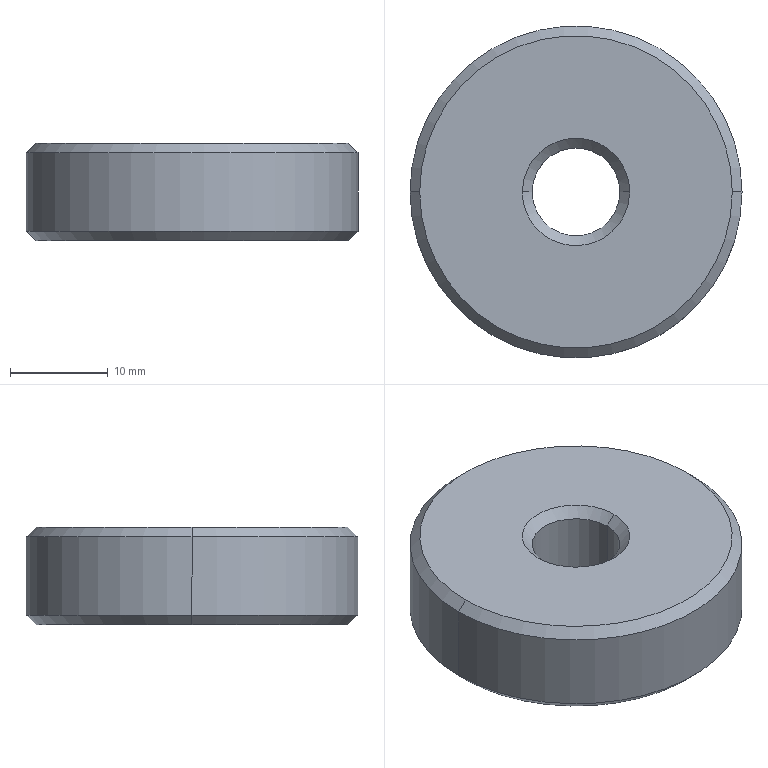Part | STEP file | 101000007785 | 1 solid | 14 faces | box 34 x 34 x 10 mm | volume 8308 mm3 | cone 8 | cylinder 4 | plane 2 | commonest cylinder face diameters 9 x2 34 x2
STEP:
#1=CARTESIAN_POINT('',(16.,0.,10.));
#2=VERTEX_POINT('',#1);
#3=CARTESIAN_POINT('',(-16.,0.,10.));
#4=VERTEX_POINT('',#3);
#5=CARTESIAN_POINT('',(0.,0.,10.));
#6=DIRECTION('',(0.,0.,-1.));
#7=AXIS2_PLACEMENT_3D('',#5,#6,$);
#8=CIRCLE('',#7,16.);
#9=EDGE_CURVE('',#2,#4,#8,.F.);
#10=ORIENTED_EDGE('',*,*,#9,.F.);
#11=CARTESIAN_POINT('',(17.,0.,9.));
#12=VERTEX_POINT('',#11);
#13=CARTESIAN_POINT('',(353561.391,0.,-353535.391));
#14=DIRECTION('',(0.7071,0.,-0.7071));
#15=VECTOR('',#14,1.);
#16=LINE('',#13,#15);
#17=EDGE_CURVE('',#2,#12,#16,.T.);
#18=ORIENTED_EDGE('',*,*,#17,.T.);
#19=CARTESIAN_POINT('',(-17.,0.,9.));
#20=VERTEX_POINT('',#19);
#21=CARTESIAN_POINT('',(0.,0.,9.));
#22=DIRECTION('',(0.,0.,-1.));
#23=AXIS2_PLACEMENT_3D('',#21,#22,$);
#24=CIRCLE('',#23,17.);
#25=EDGE_CURVE('',#20,#12,#24,.T.);
#26=ORIENTED_EDGE('',*,*,#25,.F.);
#27=CARTESIAN_POINT('',(-353561.391,0.,-353535.391));
#28=DIRECTION('',(-0.7071,0.,-0.7071));
#29=VECTOR('',#28,1.);
#30=LINE('',#27,#29);
#31=EDGE_CURVE('',#4,#20,#30,.T.);
#32=ORIENTED_EDGE('',*,*,#31,.F.);
#33=EDGE_LOOP('',(#10,#18,#26,#32));
#34=FACE_OUTER_BOUND('',#33,.T.);
#35=CARTESIAN_POINT('',(0.,0.,10.));
#36=DIRECTION('',(0.,0.,-1.));
#37=DIRECTION('',(-1.,0.,0.));
#38=AXIS2_PLACEMENT_3D('',#35,#36,#37);
#39=CONICAL_SURFACE('',#38,16.,0.7854);
#40=ADVANCED_FACE('',(#34),#39,.T.);
#41=CARTESIAN_POINT('',(0.,0.,10.));
#42=DIRECTION('',(0.,0.,1.));
#43=AXIS2_PLACEMENT_3D('',#41,#42,$);
#44=CIRCLE('',#43,16.);
#45=EDGE_CURVE('',#4,#2,#44,.T.);
#46=ORIENTED_EDGE('',*,*,#45,.T.);
#47=ORIENTED_EDGE('',*,*,#9,.T.);
#48=EDGE_LOOP('',(#46,#47));
#49=FACE_OUTER_BOUND('',#48,.T.);
#50=CARTESIAN_POINT('',(5.5,0.,10.));
#51=VERTEX_POINT('',#50);
#52=CARTESIAN_POINT('',(-5.5,0.,10.));
#53=VERTEX_POINT('',#52);
#54=CARTESIAN_POINT('',(5.5,0.,10.));
#55=CARTESIAN_POINT('',(5.5,-0.5744,10.));
#56=CARTESIAN_POINT('',(5.425,-1.149,10.));
#57=CARTESIAN_POINT('',(5.275,-1.71,10.));
#58=CARTESIAN_POINT('',(4.832,-2.781,10.));
#59=CARTESIAN_POINT('',(4.129,-3.702,10.));
#60=CARTESIAN_POINT('',(3.719,-4.114,10.));
#61=CARTESIAN_POINT('',(2.801,-4.82,10.));
#62=CARTESIAN_POINT('',(1.732,-5.268,10.));
#63=CARTESIAN_POINT('',(1.171,-5.42,10.));
#64=CARTESIAN_POINT('',(0.02284,-5.575,10.));
#65=CARTESIAN_POINT('',(-1.127,-5.43,10.));
#66=CARTESIAN_POINT('',(-1.689,-5.282,10.));
#67=CARTESIAN_POINT('',(-2.761,-4.843,10.));
#68=CARTESIAN_POINT('',(-3.685,-4.144,10.));
#69=CARTESIAN_POINT('',(-4.098,-3.736,10.));
#70=CARTESIAN_POINT('',(-4.809,-2.82,10.));
#71=CARTESIAN_POINT('',(-5.261,-1.753,10.));
#72=CARTESIAN_POINT('',(-5.415,-1.193,10.));
#73=CARTESIAN_POINT('',(-5.496,-0.6105,10.));
#74=CARTESIAN_POINT('',(-5.5,-0.02704,10.));
#75=CARTESIAN_POINT('',(-5.5,-0.01803,10.));
#76=CARTESIAN_POINT('',(-5.5,-0.009014,10.));
#77=CARTESIAN_POINT('',(-5.5,0.,10.));
#78=B_SPLINE_CURVE_WITH_KNOTS('',5,(#54,#55,#56,#57,#58,#59,#60,#61,#62,#63,#64,#65,#66,#67,#68,#69,#70,#71,#72,#73,#74,#75,#76,#77),.UNSPECIFIED.,.F.,.U.,(6,3,3,3,3,3,3,6),(0.,4.062,8.124,12.186,16.248,20.31,24.372,24.436),.UNSPECIFIED.);
#79=EDGE_CURVE('',#51,#53,#78,.T.);
#80=ORIENTED_EDGE('',*,*,#79,.T.);
#81=CARTESIAN_POINT('',(-5.5,0.,10.));
#82=CARTESIAN_POINT('',(-5.5,0.5744,10.));
#83=CARTESIAN_POINT('',(-5.425,1.149,10.));
#84=CARTESIAN_POINT('',(-5.275,1.71,10.));
#85=CARTESIAN_POINT('',(-4.832,2.781,10.));
#86=CARTESIAN_POINT('',(-4.129,3.702,10.));
#87=CARTESIAN_POINT('',(-3.719,4.114,10.));
#88=CARTESIAN_POINT('',(-2.801,4.82,10.));
#89=CARTESIAN_POINT('',(-1.732,5.268,10.));
#90=CARTESIAN_POINT('',(-1.171,5.42,10.));
#91=CARTESIAN_POINT('',(-0.02284,5.575,10.));
#92=CARTESIAN_POINT('',(1.127,5.43,10.));
#93=CARTESIAN_POINT('',(1.689,5.282,10.));
#94=CARTESIAN_POINT('',(2.761,4.843,10.));
#95=CARTESIAN_POINT('',(3.685,4.144,10.));
#96=CARTESIAN_POINT('',(4.098,3.736,10.));
#97=CARTESIAN_POINT('',(4.809,2.82,10.));
#98=CARTESIAN_POINT('',(5.261,1.753,10.));
#99=CARTESIAN_POINT('',(5.415,1.193,10.));
#100=CARTESIAN_POINT('',(5.496,0.6105,10.));
#101=CARTESIAN_POINT('',(5.5,0.02704,10.));
#102=CARTESIAN_POINT('',(5.5,0.01803,10.));
#103=CARTESIAN_POINT('',(5.5,0.009014,10.));
#104=CARTESIAN_POINT('',(5.5,0.,10.));
#105=B_SPLINE_CURVE_WITH_KNOTS('',5,(#81,#82,#83,#84,#85,#86,#87,#88,#89,#90,#91,#92,#93,#94,#95,#96,#97,#98,#99,#100,#101,#102,#103,#104),.UNSPECIFIED.,.F.,.U.,(6,3,3,3,3,3,3,6),(0.,4.062,8.124,12.186,16.248,20.31,24.372,24.436),.UNSPECIFIED.);
#106=EDGE_CURVE('',#53,#51,#105,.T.);
#107=ORIENTED_EDGE('',*,*,#106,.T.);
#108=EDGE_LOOP('',(#80,#107));
#109=FACE_BOUND('',#108,.T.);
#110=CARTESIAN_POINT('',(0.,0.,10.));
#111=DIRECTION('',(0.,0.,1.));
#112=DIRECTION('',(1.,0.,0.));
#113=AXIS2_PLACEMENT_3D('',#110,#111,#112);
#114=PLANE('',#113);
#115=ADVANCED_FACE('',(#49,#109),#114,.T.);
#116=ORIENTED_EDGE('',*,*,#17,.F.);
#117=ORIENTED_EDGE('',*,*,#45,.F.);
#118=ORIENTED_EDGE('',*,*,#31,.T.);
#119=CARTESIAN_POINT('',(0.,0.,9.));
#120=DIRECTION('',(0.,0.,-1.));
#121=AXIS2_PLACEMENT_3D('',#119,#120,$);
#122=CIRCLE('',#121,17.);
#123=EDGE_CURVE('',#12,#20,#122,.T.);
#124=ORIENTED_EDGE('',*,*,#123,.F.);
#125=EDGE_LOOP('',(#116,#117,#118,#124));
#126=FACE_OUTER_BOUND('',#125,.T.);
#127=CARTESIAN_POINT('',(0.,0.,10.));
#128=DIRECTION('',(0.,0.,-1.));
#129=DIRECTION('',(1.,0.,0.));
#130=AXIS2_PLACEMENT_3D('',#127,#128,#129);
#131=CONICAL_SURFACE('',#130,16.,0.7854);
#132=ADVANCED_FACE('',(#126),#131,.T.);
#133=ORIENTED_EDGE('',*,*,#25,.T.);
#134=CARTESIAN_POINT('',(17.,0.,1.));
#135=VERTEX_POINT('',#134);
#136=CARTESIAN_POINT('',(17.,0.,10.));
#137=DIRECTION('',(0.,0.,-1.));
#138=VECTOR('',#137,1.);
#139=LINE('',#136,#138);
#140=EDGE_CURVE('',#12,#135,#139,.T.);
#141=ORIENTED_EDGE('',*,*,#140,.T.);
#142=CARTESIAN_POINT('',(-17.,0.,1.));
#143=VERTEX_POINT('',#142);
#144=CARTESIAN_POINT('',(0.,0.,1.));
#145=DIRECTION('',(0.,0.,-1.));
#146=AXIS2_PLACEMENT_3D('',#144,#145,$);
#147=CIRCLE('',#146,17.);
#148=EDGE_CURVE('',#135,#143,#147,.F.);
#149=ORIENTED_EDGE('',*,*,#148,.T.);
#150=CARTESIAN_POINT('',(-17.,0.,10.));
#151=DIRECTION('',(0.,0.,-1.));
#152=VECTOR('',#151,1.);
#153=LINE('',#150,#152);
#154=EDGE_CURVE('',#20,#143,#153,.T.);
#155=ORIENTED_EDGE('',*,*,#154,.F.);
#156=EDGE_LOOP('',(#133,#141,#149,#155));
#157=FACE_OUTER_BOUND('',#156,.T.);
#158=CARTESIAN_POINT('',(0.,0.,10.));
#159=DIRECTION('',(0.,0.,-1.));
#160=DIRECTION('',(-1.,0.,0.));
#161=AXIS2_PLACEMENT_3D('',#158,#159,#160);
#162=CYLINDRICAL_SURFACE('',#161,17.);
#163=ADVANCED_FACE('',(#157),#162,.T.);
#164=CARTESIAN_POINT('',(-4.5,0.,9.));
#165=VERTEX_POINT('',#164);
#166=CARTESIAN_POINT('',(4.5,0.,9.));
#167=VERTEX_POINT('',#166);
#168=CARTESIAN_POINT('',(0.,0.,9.));
#169=DIRECTION('',(0.,0.,1.));
#170=AXIS2_PLACEMENT_3D('',#168,#169,$);
#171=CIRCLE('',#170,4.5);
#172=EDGE_CURVE('',#165,#167,#171,.T.);
#173=ORIENTED_EDGE('',*,*,#172,.F.);
#174=CARTESIAN_POINT('',(-353555.641,0.,353560.141));
#175=DIRECTION('',(-0.7071,0.,0.7071));
#176=VECTOR('',#175,1.);
#177=LINE('',#174,#176);
#178=EDGE_CURVE('',#165,#53,#177,.T.);
#179=ORIENTED_EDGE('',*,*,#178,.T.);
#180=ORIENTED_EDGE('',*,*,#79,.F.);
#181=CARTESIAN_POINT('',(353555.641,0.,353560.141));
#182=DIRECTION('',(0.7071,0.,0.7071));
#183=VECTOR('',#182,1.);
#184=LINE('',#181,#183);
#185=EDGE_CURVE('',#167,#51,#184,.T.);
#186=ORIENTED_EDGE('',*,*,#185,.F.);
#187=EDGE_LOOP('',(#173,#179,#180,#186));
#188=FACE_OUTER_BOUND('',#187,.T.);
#189=CARTESIAN_POINT('',(0.,0.,9.));
#190=DIRECTION('',(0.,0.,1.));
#191=DIRECTION('',(-1.,0.,0.));
#192=AXIS2_PLACEMENT_3D('',#189,#190,#191);
#193=CONICAL_SURFACE('',#192,4.5,0.7854);
#194=ADVANCED_FACE('',(#188),#193,.F.);
#195=ORIENTED_EDGE('',*,*,#178,.F.);
#196=CARTESIAN_POINT('',(0.,0.,9.));
#197=DIRECTION('',(0.,0.,1.));
#198=AXIS2_PLACEMENT_3D('',#196,#197,$);
#199=CIRCLE('',#198,4.5);
#200=EDGE_CURVE('',#167,#165,#199,.T.);
#201=ORIENTED_EDGE('',*,*,#200,.F.);
#202=ORIENTED_EDGE('',*,*,#185,.T.);
#203=ORIENTED_EDGE('',*,*,#106,.F.);
#204=EDGE_LOOP('',(#195,#201,#202,#203));
#205=FACE_OUTER_BOUND('',#204,.T.);
#206=CARTESIAN_POINT('',(0.,0.,9.));
#207=DIRECTION('',(0.,0.,1.));
#208=DIRECTION('',(1.,0.,0.));
#209=AXIS2_PLACEMENT_3D('',#206,#207,#208);
#210=CONICAL_SURFACE('',#209,4.5,0.7854);
#211=ADVANCED_FACE('',(#205),#210,.F.);
#212=ORIENTED_EDGE('',*,*,#140,.F.);
#213=ORIENTED_EDGE('',*,*,#123,.T.);
#214=ORIENTED_EDGE('',*,*,#154,.T.);
#215=CARTESIAN_POINT('',(0.,0.,1.));
#216=DIRECTION('',(0.,0.,-1.));
#217=AXIS2_PLACEMENT_3D('',#215,#216,$);
#218=CIRCLE('',#217,17.);
#219=EDGE_CURVE('',#143,#135,#218,.F.);
#220=ORIENTED_EDGE('',*,*,#219,.T.);
#221=EDGE_LOOP('',(#212,#213,#214,#220));
#222=FACE_OUTER_BOUND('',#221,.T.);
#223=CARTESIAN_POINT('',(0.,0.,10.));
#224=DIRECTION('',(0.,0.,-1.));
#225=DIRECTION('',(1.,0.,0.));
#226=AXIS2_PLACEMENT_3D('',#223,#224,#225);
#227=CYLINDRICAL_SURFACE('',#226,17.);
#228=ADVANCED_FACE('',(#222),#227,.T.);
#229=CARTESIAN_POINT('',(-16.,0.,0.));
#230=VERTEX_POINT('',#229);
#231=CARTESIAN_POINT('',(16.,0.,0.));
#232=VERTEX_POINT('',#231);
#233=CARTESIAN_POINT('',(0.,0.,0.));
#234=DIRECTION('',(0.,0.,1.));
#235=AXIS2_PLACEMENT_3D('',#233,#234,$);
#236=CIRCLE('',#235,16.);
#237=EDGE_CURVE('',#230,#232,#236,.F.);
#238=ORIENTED_EDGE('',*,*,#237,.F.);
#239=CARTESIAN_POINT('',(-353561.891,0.,353545.891));
#240=DIRECTION('',(-0.7071,0.,0.7071));
#241=VECTOR('',#240,1.);
#242=LINE('',#239,#241);
#243=EDGE_CURVE('',#230,#143,#242,.T.);
#244=ORIENTED_EDGE('',*,*,#243,.T.);
#245=ORIENTED_EDGE('',*,*,#148,.F.);
#246=CARTESIAN_POINT('',(353561.891,0.,353545.891));
#247=DIRECTION('',(0.7071,0.,0.7071));
#248=VECTOR('',#247,1.);
#249=LINE('',#246,#248);
#250=EDGE_CURVE('',#232,#135,#249,.T.);
#251=ORIENTED_EDGE('',*,*,#250,.F.);
#252=EDGE_LOOP('',(#238,#244,#245,#251));
#253=FACE_OUTER_BOUND('',#252,.T.);
#254=CARTESIAN_POINT('',(0.,0.,1.));
#255=DIRECTION('',(0.,0.,1.));
#256=DIRECTION('',(1.,0.,0.));
#257=AXIS2_PLACEMENT_3D('',#254,#255,#256);
#258=CONICAL_SURFACE('',#257,17.,0.7854);
#259=ADVANCED_FACE('',(#253),#258,.T.);
#260=ORIENTED_EDGE('',*,*,#172,.T.);
#261=CARTESIAN_POINT('',(4.5,0.,1.));
#262=VERTEX_POINT('',#261);
#263=CARTESIAN_POINT('',(4.5,0.,10.));
#264=DIRECTION('',(0.,0.,-1.));
#265=VECTOR('',#264,1.);
#266=LINE('',#263,#265);
#267=EDGE_CURVE('',#167,#262,#266,.T.);
#268=ORIENTED_EDGE('',*,*,#267,.T.);
#269=CARTESIAN_POINT('',(-4.5,0.,1.));
#270=VERTEX_POINT('',#269);
#271=CARTESIAN_POINT('',(0.,0.,1.));
#272=DIRECTION('',(0.,0.,-1.));
#273=AXIS2_PLACEMENT_3D('',#271,#272,$);
#274=CIRCLE('',#273,4.5);
#275=EDGE_CURVE('',#262,#270,#274,.T.);
#276=ORIENTED_EDGE('',*,*,#275,.T.);
#277=CARTESIAN_POINT('',(-4.5,0.,10.));
#278=DIRECTION('',(0.,0.,-1.));
#279=VECTOR('',#278,1.);
#280=LINE('',#277,#279);
#281=EDGE_CURVE('',#165,#270,#280,.T.);
#282=ORIENTED_EDGE('',*,*,#281,.F.);
#283=EDGE_LOOP('',(#260,#268,#276,#282));
#284=FACE_OUTER_BOUND('',#283,.T.);
#285=CARTESIAN_POINT('',(0.,0.,10.));
#286=DIRECTION('',(0.,0.,-1.));
#287=DIRECTION('',(1.,0.,0.));
#288=AXIS2_PLACEMENT_3D('',#285,#286,#287);
#289=CYLINDRICAL_SURFACE('',#288,4.5);
#290=ADVANCED_FACE('',(#284),#289,.F.);
#291=ORIENTED_EDGE('',*,*,#267,.F.);
#292=ORIENTED_EDGE('',*,*,#200,.T.);
#293=ORIENTED_EDGE('',*,*,#281,.T.);
#294=CARTESIAN_POINT('',(0.,0.,1.));
#295=DIRECTION('',(0.,0.,-1.));
#296=AXIS2_PLACEMENT_3D('',#294,#295,$);
#297=CIRCLE('',#296,4.5);
#298=EDGE_CURVE('',#270,#262,#297,.T.);
#299=ORIENTED_EDGE('',*,*,#298,.T.);
#300=EDGE_LOOP('',(#291,#292,#293,#299));
#301=FACE_OUTER_BOUND('',#300,.T.);
#302=CARTESIAN_POINT('',(0.,0.,10.));
#303=DIRECTION('',(0.,0.,-1.));
#304=DIRECTION('',(-1.,0.,0.));
#305=AXIS2_PLACEMENT_3D('',#302,#303,#304);
#306=CYLINDRICAL_SURFACE('',#305,4.5);
#307=ADVANCED_FACE('',(#301),#306,.F.);
#308=ORIENTED_EDGE('',*,*,#243,.F.);
#309=CARTESIAN_POINT('',(0.,0.,0.));
#310=DIRECTION('',(0.,0.,1.));
#311=AXIS2_PLACEMENT_3D('',#309,#310,$);
#312=CIRCLE('',#311,16.);
#313=EDGE_CURVE('',#232,#230,#312,.F.);
#314=ORIENTED_EDGE('',*,*,#313,.F.);
#315=ORIENTED_EDGE('',*,*,#250,.T.);
#316=ORIENTED_EDGE('',*,*,#219,.F.);
#317=EDGE_LOOP('',(#308,#314,#315,#316));
#318=FACE_OUTER_BOUND('',#317,.T.);
#319=CARTESIAN_POINT('',(0.,0.,1.));
#320=DIRECTION('',(0.,0.,1.));
#321=DIRECTION('',(-1.,0.,0.));
#322=AXIS2_PLACEMENT_3D('',#319,#320,#321);
#323=CONICAL_SURFACE('',#322,17.,0.7854);
#324=ADVANCED_FACE('',(#318),#323,.T.);
#325=ORIENTED_EDGE('',*,*,#313,.T.);
#326=ORIENTED_EDGE('',*,*,#237,.T.);
#327=EDGE_LOOP('',(#325,#326));
#328=FACE_OUTER_BOUND('',#327,.T.);
#329=CARTESIAN_POINT('',(-5.5,0.,0.));
#330=VERTEX_POINT('',#329);
#331=CARTESIAN_POINT('',(5.5,0.,0.));
#332=VERTEX_POINT('',#331);
#333=CARTESIAN_POINT('',(0.,0.,0.));
#334=DIRECTION('',(0.,0.,1.));
#335=AXIS2_PLACEMENT_3D('',#333,#334,$);
#336=CIRCLE('',#335,5.5);
#337=EDGE_CURVE('',#330,#332,#336,.T.);
#338=ORIENTED_EDGE('',*,*,#337,.T.);
#339=CARTESIAN_POINT('',(0.,0.,0.));
#340=DIRECTION('',(0.,0.,1.));
#341=AXIS2_PLACEMENT_3D('',#339,#340,$);
#342=CIRCLE('',#341,5.5);
#343=EDGE_CURVE('',#332,#330,#342,.T.);
#344=ORIENTED_EDGE('',*,*,#343,.T.);
#345=EDGE_LOOP('',(#338,#344));
#346=FACE_BOUND('',#345,.T.);
#347=CARTESIAN_POINT('',(0.,0.,0.));
#348=DIRECTION('',(0.,0.,1.));
#349=DIRECTION('',(1.,0.,0.));
#350=AXIS2_PLACEMENT_3D('',#347,#348,#349);
#351=PLANE('',#350);
#352=ADVANCED_FACE('',(#328,#346),#351,.F.);
#353=ORIENTED_EDGE('',*,*,#275,.F.);
#354=CARTESIAN_POINT('',(353556.141,0.,-353550.641));
#355=DIRECTION('',(0.7071,0.,-0.7071));
#356=VECTOR('',#355,1.);
#357=LINE('',#354,#356);
#358=EDGE_CURVE('',#262,#332,#357,.T.);
#359=ORIENTED_EDGE('',*,*,#358,.T.);
#360=ORIENTED_EDGE('',*,*,#337,.F.);
#361=CARTESIAN_POINT('',(-353556.141,0.,-353550.641));
#362=DIRECTION('',(-0.7071,0.,-0.7071));
#363=VECTOR('',#362,1.);
#364=LINE('',#361,#363);
#365=EDGE_CURVE('',#270,#330,#364,.T.);
#366=ORIENTED_EDGE('',*,*,#365,.F.);
#367=EDGE_LOOP('',(#353,#359,#360,#366));
#368=FACE_OUTER_BOUND('',#367,.T.);
#369=CARTESIAN_POINT('',(0.,0.,0.));
#370=DIRECTION('',(0.,0.,-1.));
#371=DIRECTION('',(1.,0.,0.));
#372=AXIS2_PLACEMENT_3D('',#369,#370,#371);
#373=CONICAL_SURFACE('',#372,5.5,0.7854);
#374=ADVANCED_FACE('',(#368),#373,.F.);
#375=ORIENTED_EDGE('',*,*,#358,.F.);
#376=ORIENTED_EDGE('',*,*,#298,.F.);
#377=ORIENTED_EDGE('',*,*,#365,.T.);
#378=ORIENTED_EDGE('',*,*,#343,.F.);
#379=EDGE_LOOP('',(#375,#376,#377,#378));
#380=FACE_OUTER_BOUND('',#379,.T.);
#381=CARTESIAN_POINT('',(0.,0.,0.));
#382=DIRECTION('',(0.,0.,-1.));
#383=DIRECTION('',(-1.,0.,0.));
#384=AXIS2_PLACEMENT_3D('',#381,#382,#383);
#385=CONICAL_SURFACE('',#384,5.5,0.7854);
#386=ADVANCED_FACE('',(#380),#385,.F.);
#387=CLOSED_SHELL('',(#40,#115,#132,#163,#194,#211,#228,#259,#290,#307,#324,#352,#374,#386));
#388=MANIFOLD_SOLID_BREP('',#387);
#389=(LENGTH_UNIT()NAMED_UNIT(*)SI_UNIT(.MILLI.,.METRE.));
#390=UNCERTAINTY_MEASURE_WITH_UNIT(LENGTH_MEASURE(0.005),#389,'','');
#391=(NAMED_UNIT(*)PLANE_ANGLE_UNIT()SI_UNIT($,.RADIAN.));
#392=(NAMED_UNIT(*)SI_UNIT($,.STERADIAN.)SOLID_ANGLE_UNIT());
#393=(GEOMETRIC_REPRESENTATION_CONTEXT(3)GLOBAL_UNCERTAINTY_ASSIGNED_CONTEXT((#390))GLOBAL_UNIT_ASSIGNED_CONTEXT((#389,#391,#392))REPRESENTATION_CONTEXT('',''));
#394=ADVANCED_BREP_SHAPE_REPRESENTATION('',(#388),#393);